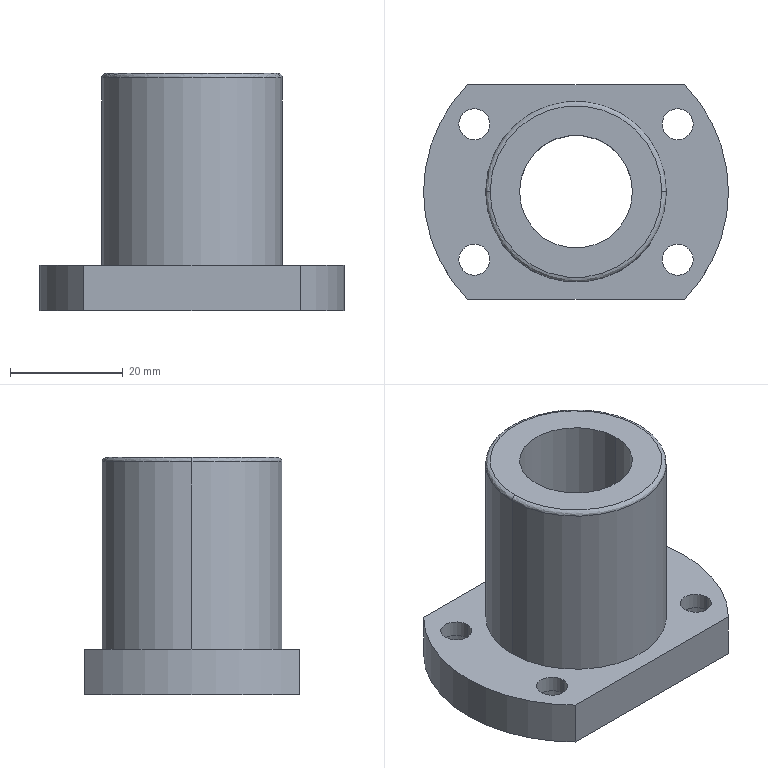Part | SolidWorks | features BaseBody 1 | 1 solid | 34 faces | box 54 x 38 x 42 mm | volume 27501 mm3 | cylinder 23 | plane 9 | spline 2 | commonest cylinder face diameters 5.5 x8 9 x8 54 x3 20 x2 32 x2
STEP:
#1=CARTESIAN_POINT('',(16.,0.,41.2));
#2=VERTEX_POINT('',#1);
#3=CARTESIAN_POINT('',(-16.,0.,41.2));
#4=VERTEX_POINT('',#3);
#5=CARTESIAN_POINT('',(0.,0.,41.2));
#6=DIRECTION('',(0.,0.,-1.));
#7=DIRECTION('',(1.,0.,0.));
#8=AXIS2_PLACEMENT_3D('',#5,#6,#7);
#9=CIRCLE('',#8,16.);
#10=EDGE_CURVE('',#2,#4,#9,.T.);
#11=ORIENTED_EDGE('',*,*,#10,.F.);
#12=CARTESIAN_POINT('',(15.2,0.,42.));
#13=VERTEX_POINT('',#12);
#14=CARTESIAN_POINT('',(15.2,0.,41.2));
#15=DIRECTION('',(0.,-1.,0.));
#16=DIRECTION('',(1.,0.,0.));
#17=AXIS2_PLACEMENT_3D('',#14,#15,#16);
#18=CIRCLE('',#17,0.8);
#19=EDGE_CURVE('',#2,#13,#18,.T.);
#20=ORIENTED_EDGE('',*,*,#19,.T.);
#21=CARTESIAN_POINT('',(-15.2,0.,42.));
#22=VERTEX_POINT('',#21);
#23=CARTESIAN_POINT('',(15.2,0.,42.));
#24=CARTESIAN_POINT('',(15.2,-30.4,42.));
#25=CARTESIAN_POINT('',(-15.2,-30.4,42.));
#26=CARTESIAN_POINT('',(-15.2,0.,42.));
#27=(BOUNDED_CURVE()B_SPLINE_CURVE(3,(#23,#24,#25,#26),.UNSPECIFIED.,.F.,.F.)B_SPLINE_CURVE_WITH_KNOTS((4,4),(0.5,1.),.UNSPECIFIED.)CURVE()GEOMETRIC_REPRESENTATION_ITEM()RATIONAL_B_SPLINE_CURVE((1.,0.3333,0.3333,1.))REPRESENTATION_ITEM(''));
#28=EDGE_CURVE('',#13,#22,#27,.T.);
#29=ORIENTED_EDGE('',*,*,#28,.T.);
#30=CARTESIAN_POINT('',(-15.2,0.,41.2));
#31=DIRECTION('',(0.,1.,0.));
#32=DIRECTION('',(-1.,0.,0.));
#33=AXIS2_PLACEMENT_3D('',#30,#31,#32);
#34=CIRCLE('',#33,0.8);
#35=EDGE_CURVE('',#4,#22,#34,.T.);
#36=ORIENTED_EDGE('',*,*,#35,.F.);
#37=EDGE_LOOP('',(#11,#20,#29,#36));
#38=FACE_OUTER_BOUND('',#37,.T.);
#39=CARTESIAN_POINT('',(16.,0.,41.2));
#40=CARTESIAN_POINT('',(16.,-32.,41.2));
#41=CARTESIAN_POINT('',(-16.,-32.,41.2));
#42=CARTESIAN_POINT('',(-16.,0.,41.2));
#43=CARTESIAN_POINT('',(16.,0.,41.669));
#44=CARTESIAN_POINT('',(16.,-32.,41.669));
#45=CARTESIAN_POINT('',(-16.,-32.,41.669));
#46=CARTESIAN_POINT('',(-16.,0.,41.669));
#47=CARTESIAN_POINT('',(15.669,0.,42.));
#48=CARTESIAN_POINT('',(15.669,-31.337,42.));
#49=CARTESIAN_POINT('',(-15.669,-31.337,42.));
#50=CARTESIAN_POINT('',(-15.669,0.,42.));
#51=CARTESIAN_POINT('',(15.2,0.,42.));
#52=CARTESIAN_POINT('',(15.2,-30.4,42.));
#53=CARTESIAN_POINT('',(-15.2,-30.4,42.));
#54=CARTESIAN_POINT('',(-15.2,0.,42.));
#55=(BOUNDED_SURFACE()B_SPLINE_SURFACE(3,3,((#39,#40,#41,#42),(#43,#44,#45,#46),(#47,#48,#49,#50),(#51,#52,#53,#54)),.UNSPECIFIED.,.F.,.F.,.F.)B_SPLINE_SURFACE_WITH_KNOTS((4,4),(4,4),(0.,1.),(0.,1.),.UNSPECIFIED.)GEOMETRIC_REPRESENTATION_ITEM()RATIONAL_B_SPLINE_SURFACE(((1.,0.3333,0.3333,1.),(0.8047,0.2682,0.2682,0.8047),(0.8047,0.2682,0.2682,0.8047),(1.,0.3333,0.3333,1.)))REPRESENTATION_ITEM('')SURFACE());
#56=ADVANCED_FACE('',(#38),#55,.T.);
#57=CARTESIAN_POINT('',(16.,0.,8.));
#58=VERTEX_POINT('',#57);
#59=CARTESIAN_POINT('',(-16.,0.,8.));
#60=VERTEX_POINT('',#59);
#61=CARTESIAN_POINT('',(0.,0.,8.));
#62=DIRECTION('',(0.,0.,1.));
#63=DIRECTION('',(1.,0.,0.));
#64=AXIS2_PLACEMENT_3D('',#61,#62,#63);
#65=CIRCLE('',#64,16.);
#66=EDGE_CURVE('',#58,#60,#65,.T.);
#67=ORIENTED_EDGE('',*,*,#66,.T.);
#68=CARTESIAN_POINT('',(-16.,0.,0.));
#69=DIRECTION('',(0.,0.,1.));
#70=VECTOR('',#69,1000.);
#71=LINE('',#68,#70);
#72=EDGE_CURVE('',#60,#4,#71,.T.);
#73=ORIENTED_EDGE('',*,*,#72,.T.);
#74=CARTESIAN_POINT('',(0.,0.,41.2));
#75=DIRECTION('',(0.,0.,-1.));
#76=DIRECTION('',(1.,0.,0.));
#77=AXIS2_PLACEMENT_3D('',#74,#75,#76);
#78=CIRCLE('',#77,16.);
#79=EDGE_CURVE('',#4,#2,#78,.T.);
#80=ORIENTED_EDGE('',*,*,#79,.T.);
#81=CARTESIAN_POINT('',(16.,0.,0.));
#82=DIRECTION('',(0.,0.,1.));
#83=VECTOR('',#82,1000.);
#84=LINE('',#81,#83);
#85=EDGE_CURVE('',#58,#2,#84,.T.);
#86=ORIENTED_EDGE('',*,*,#85,.F.);
#87=EDGE_LOOP('',(#67,#73,#80,#86));
#88=FACE_OUTER_BOUND('',#87,.T.);
#89=CARTESIAN_POINT('',(0.,0.,0.));
#90=DIRECTION('',(0.,0.,1.));
#91=DIRECTION('',(1.,0.,0.));
#92=AXIS2_PLACEMENT_3D('',#89,#90,#91);
#93=CYLINDRICAL_SURFACE('',#92,16.);
#94=ADVANCED_FACE('',(#88),#93,.T.);
#95=CARTESIAN_POINT('',(19.183,-19.,0.));
#96=VERTEX_POINT('',#95);
#97=CARTESIAN_POINT('',(27.,0.,0.));
#98=VERTEX_POINT('',#97);
#99=CARTESIAN_POINT('',(0.,0.,0.));
#100=DIRECTION('',(0.,0.,1.));
#101=DIRECTION('',(1.,0.,0.));
#102=AXIS2_PLACEMENT_3D('',#99,#100,#101);
#103=CIRCLE('',#102,27.);
#104=EDGE_CURVE('',#96,#98,#103,.T.);
#105=ORIENTED_EDGE('',*,*,#104,.T.);
#106=CARTESIAN_POINT('',(27.,0.,8.));
#107=VERTEX_POINT('',#106);
#108=CARTESIAN_POINT('',(27.,0.,8.));
#109=DIRECTION('',(0.,0.,1.));
#110=VECTOR('',#109,1000.);
#111=LINE('',#108,#110);
#112=EDGE_CURVE('',#98,#107,#111,.T.);
#113=ORIENTED_EDGE('',*,*,#112,.T.);
#114=CARTESIAN_POINT('',(19.183,-19.,8.));
#115=VERTEX_POINT('',#114);
#116=CARTESIAN_POINT('',(0.,0.,8.));
#117=DIRECTION('',(0.,0.,1.));
#118=DIRECTION('',(1.,0.,0.));
#119=AXIS2_PLACEMENT_3D('',#116,#117,#118);
#120=CIRCLE('',#119,27.);
#121=EDGE_CURVE('',#115,#107,#120,.T.);
#122=ORIENTED_EDGE('',*,*,#121,.F.);
#123=CARTESIAN_POINT('',(19.183,-19.,8.));
#124=DIRECTION('',(0.,0.,-1.));
#125=VECTOR('',#124,1000.);
#126=LINE('',#123,#125);
#127=EDGE_CURVE('',#115,#96,#126,.T.);
#128=ORIENTED_EDGE('',*,*,#127,.T.);
#129=EDGE_LOOP('',(#105,#113,#122,#128));
#130=FACE_OUTER_BOUND('',#129,.T.);
#131=CARTESIAN_POINT('',(0.,0.,8.));
#132=DIRECTION('',(0.,0.,1.));
#133=DIRECTION('',(1.,0.,0.));
#134=AXIS2_PLACEMENT_3D('',#131,#132,#133);
#135=CYLINDRICAL_SURFACE('',#134,27.);
#136=ADVANCED_FACE('',(#130),#135,.T.);
#137=CARTESIAN_POINT('',(-20.75,-12.,5.1));
#138=VERTEX_POINT('',#137);
#139=CARTESIAN_POINT('',(-15.25,-12.,5.1));
#140=VERTEX_POINT('',#139);
#141=CARTESIAN_POINT('',(-18.,-12.,5.1));
#142=DIRECTION('',(0.,0.,1.));
#143=DIRECTION('',(1.,0.,0.));
#144=AXIS2_PLACEMENT_3D('',#141,#142,#143);
#145=CIRCLE('',#144,2.75);
#146=EDGE_CURVE('',#138,#140,#145,.T.);
#147=ORIENTED_EDGE('',*,*,#146,.F.);
#148=CARTESIAN_POINT('',(-20.75,-12.,8.));
#149=VERTEX_POINT('',#148);
#150=CARTESIAN_POINT('',(-20.75,-12.,0.));
#151=DIRECTION('',(0.,0.,1.));
#152=VECTOR('',#151,1000.);
#153=LINE('',#150,#152);
#154=EDGE_CURVE('',#138,#149,#153,.T.);
#155=ORIENTED_EDGE('',*,*,#154,.T.);
#156=CARTESIAN_POINT('',(-15.25,-12.,8.));
#157=VERTEX_POINT('',#156);
#158=CARTESIAN_POINT('',(-18.,-12.,8.));
#159=DIRECTION('',(0.,0.,-1.));
#160=DIRECTION('',(1.,0.,0.));
#161=AXIS2_PLACEMENT_3D('',#158,#159,#160);
#162=CIRCLE('',#161,2.75);
#163=EDGE_CURVE('',#157,#149,#162,.T.);
#164=ORIENTED_EDGE('',*,*,#163,.F.);
#165=CARTESIAN_POINT('',(-15.25,-12.,0.));
#166=DIRECTION('',(0.,0.,1.));
#167=VECTOR('',#166,1000.);
#168=LINE('',#165,#167);
#169=EDGE_CURVE('',#140,#157,#168,.T.);
#170=ORIENTED_EDGE('',*,*,#169,.F.);
#171=EDGE_LOOP('',(#147,#155,#164,#170));
#172=FACE_OUTER_BOUND('',#171,.T.);
#173=CARTESIAN_POINT('',(-18.,-12.,0.));
#174=DIRECTION('',(0.,0.,1.));
#175=DIRECTION('',(1.,0.,0.));
#176=AXIS2_PLACEMENT_3D('',#173,#174,#175);
#177=CYLINDRICAL_SURFACE('',#176,2.75);
#178=ADVANCED_FACE('',(#172),#177,.F.);
#179=CARTESIAN_POINT('',(20.75,-12.,8.));
#180=VERTEX_POINT('',#179);
#181=CARTESIAN_POINT('',(15.25,-12.,8.));
#182=VERTEX_POINT('',#181);
#183=CARTESIAN_POINT('',(18.,-12.,8.));
#184=DIRECTION('',(0.,0.,-1.));
#185=DIRECTION('',(-1.,0.,0.));
#186=AXIS2_PLACEMENT_3D('',#183,#184,#185);
#187=CIRCLE('',#186,2.75);
#188=EDGE_CURVE('',#180,#182,#187,.T.);
#189=ORIENTED_EDGE('',*,*,#188,.F.);
#190=CARTESIAN_POINT('',(20.75,-12.,5.1));
#191=VERTEX_POINT('',#190);
#192=CARTESIAN_POINT('',(20.75,-12.,8.));
#193=DIRECTION('',(0.,0.,-1.));
#194=VECTOR('',#193,1000.);
#195=LINE('',#192,#194);
#196=EDGE_CURVE('',#180,#191,#195,.T.);
#197=ORIENTED_EDGE('',*,*,#196,.T.);
#198=CARTESIAN_POINT('',(15.25,-12.,5.1));
#199=VERTEX_POINT('',#198);
#200=CARTESIAN_POINT('',(18.,-12.,5.1));
#201=DIRECTION('',(0.,0.,1.));
#202=DIRECTION('',(-1.,0.,0.));
#203=AXIS2_PLACEMENT_3D('',#200,#201,#202);
#204=CIRCLE('',#203,2.75);
#205=EDGE_CURVE('',#199,#191,#204,.T.);
#206=ORIENTED_EDGE('',*,*,#205,.F.);
#207=CARTESIAN_POINT('',(15.25,-12.,8.));
#208=DIRECTION('',(0.,0.,-1.));
#209=VECTOR('',#208,1000.);
#210=LINE('',#207,#209);
#211=EDGE_CURVE('',#182,#199,#210,.T.);
#212=ORIENTED_EDGE('',*,*,#211,.F.);
#213=EDGE_LOOP('',(#189,#197,#206,#212));
#214=FACE_OUTER_BOUND('',#213,.T.);
#215=CARTESIAN_POINT('',(18.,-12.,8.));
#216=DIRECTION('',(0.,0.,-1.));
#217=DIRECTION('',(-1.,0.,0.));
#218=AXIS2_PLACEMENT_3D('',#215,#216,#217);
#219=CYLINDRICAL_SURFACE('',#218,2.75);
#220=ADVANCED_FACE('',(#214),#219,.F.);
#221=CARTESIAN_POINT('',(-20.75,12.,5.1));
#222=VERTEX_POINT('',#221);
#223=CARTESIAN_POINT('',(-15.25,12.,5.1));
#224=VERTEX_POINT('',#223);
#225=CARTESIAN_POINT('',(-18.,12.,5.1));
#226=DIRECTION('',(0.,0.,1.));
#227=DIRECTION('',(1.,0.,0.));
#228=AXIS2_PLACEMENT_3D('',#225,#226,#227);
#229=CIRCLE('',#228,2.75);
#230=EDGE_CURVE('',#222,#224,#229,.T.);
#231=ORIENTED_EDGE('',*,*,#230,.F.);
#232=CARTESIAN_POINT('',(-20.75,12.,8.));
#233=VERTEX_POINT('',#232);
#234=CARTESIAN_POINT('',(-20.75,12.,0.));
#235=DIRECTION('',(0.,0.,1.));
#236=VECTOR('',#235,1000.);
#237=LINE('',#234,#236);
#238=EDGE_CURVE('',#222,#233,#237,.T.);
#239=ORIENTED_EDGE('',*,*,#238,.T.);
#240=CARTESIAN_POINT('',(-15.25,12.,8.));
#241=VERTEX_POINT('',#240);
#242=CARTESIAN_POINT('',(-18.,12.,8.));
#243=DIRECTION('',(0.,0.,-1.));
#244=DIRECTION('',(1.,0.,0.));
#245=AXIS2_PLACEMENT_3D('',#242,#243,#244);
#246=CIRCLE('',#245,2.75);
#247=EDGE_CURVE('',#241,#233,#246,.T.);
#248=ORIENTED_EDGE('',*,*,#247,.F.);
#249=CARTESIAN_POINT('',(-15.25,12.,0.));
#250=DIRECTION('',(0.,0.,1.));
#251=VECTOR('',#250,1000.);
#252=LINE('',#249,#251);
#253=EDGE_CURVE('',#224,#241,#252,.T.);
#254=ORIENTED_EDGE('',*,*,#253,.F.);
#255=EDGE_LOOP('',(#231,#239,#248,#254));
#256=FACE_OUTER_BOUND('',#255,.T.);
#257=CARTESIAN_POINT('',(-18.,12.,0.));
#258=DIRECTION('',(0.,0.,1.));
#259=DIRECTION('',(1.,0.,0.));
#260=AXIS2_PLACEMENT_3D('',#257,#258,#259);
#261=CYLINDRICAL_SURFACE('',#260,2.75);
#262=ADVANCED_FACE('',(#256),#261,.F.);
#263=CARTESIAN_POINT('',(20.75,12.,8.));
#264=VERTEX_POINT('',#263);
#265=CARTESIAN_POINT('',(15.25,12.,8.));
#266=VERTEX_POINT('',#265);
#267=CARTESIAN_POINT('',(18.,12.,8.));
#268=DIRECTION('',(0.,0.,-1.));
#269=DIRECTION('',(-1.,0.,0.));
#270=AXIS2_PLACEMENT_3D('',#267,#268,#269);
#271=CIRCLE('',#270,2.75);
#272=EDGE_CURVE('',#264,#266,#271,.T.);
#273=ORIENTED_EDGE('',*,*,#272,.F.);
#274=CARTESIAN_POINT('',(20.75,12.,5.1));
#275=VERTEX_POINT('',#274);
#276=CARTESIAN_POINT('',(20.75,12.,8.));
#277=DIRECTION('',(0.,0.,-1.));
#278=VECTOR('',#277,1000.);
#279=LINE('',#276,#278);
#280=EDGE_CURVE('',#264,#275,#279,.T.);
#281=ORIENTED_EDGE('',*,*,#280,.T.);
#282=CARTESIAN_POINT('',(15.25,12.,5.1));
#283=VERTEX_POINT('',#282);
#284=CARTESIAN_POINT('',(18.,12.,5.1));
#285=DIRECTION('',(0.,0.,1.));
#286=DIRECTION('',(-1.,0.,0.));
#287=AXIS2_PLACEMENT_3D('',#284,#285,#286);
#288=CIRCLE('',#287,2.75);
#289=EDGE_CURVE('',#283,#275,#288,.T.);
#290=ORIENTED_EDGE('',*,*,#289,.F.);
#291=CARTESIAN_POINT('',(15.25,12.,8.));
#292=DIRECTION('',(0.,0.,-1.));
#293=VECTOR('',#292,1000.);
#294=LINE('',#291,#293);
#295=EDGE_CURVE('',#266,#283,#294,.T.);
#296=ORIENTED_EDGE('',*,*,#295,.F.);
#297=EDGE_LOOP('',(#273,#281,#290,#296));
#298=FACE_OUTER_BOUND('',#297,.T.);
#299=CARTESIAN_POINT('',(18.,12.,8.));
#300=DIRECTION('',(0.,0.,-1.));
#301=DIRECTION('',(-1.,0.,0.));
#302=AXIS2_PLACEMENT_3D('',#299,#300,#301);
#303=CYLINDRICAL_SURFACE('',#302,2.75);
#304=ADVANCED_FACE('',(#298),#303,.F.);
#305=CARTESIAN_POINT('',(-10.,0.,0.));
#306=VERTEX_POINT('',#305);
#307=CARTESIAN_POINT('',(10.,0.,0.));
#308=VERTEX_POINT('',#307);
#309=CARTESIAN_POINT('',(0.,0.,0.));
#310=DIRECTION('',(0.,0.,1.));
#311=DIRECTION('',(1.,0.,0.));
#312=AXIS2_PLACEMENT_3D('',#309,#310,#311);
#313=CIRCLE('',#312,10.);
#314=EDGE_CURVE('',#306,#308,#313,.T.);
#315=ORIENTED_EDGE('',*,*,#314,.F.);
#316=CARTESIAN_POINT('',(-10.,0.,42.));
#317=VERTEX_POINT('',#316);
#318=CARTESIAN_POINT('',(-10.,0.,0.));
#319=DIRECTION('',(0.,0.,1.));
#320=VECTOR('',#319,1000.);
#321=LINE('',#318,#320);
#322=EDGE_CURVE('',#306,#317,#321,.T.);
#323=ORIENTED_EDGE('',*,*,#322,.T.);
#324=CARTESIAN_POINT('',(10.,0.,42.));
#325=VERTEX_POINT('',#324);
#326=CARTESIAN_POINT('',(0.,0.,42.));
#327=DIRECTION('',(0.,0.,-1.));
#328=DIRECTION('',(1.,0.,0.));
#329=AXIS2_PLACEMENT_3D('',#326,#327,#328);
#330=CIRCLE('',#329,10.);
#331=EDGE_CURVE('',#325,#317,#330,.T.);
#332=ORIENTED_EDGE('',*,*,#331,.F.);
#333=CARTESIAN_POINT('',(10.,0.,0.));
#334=DIRECTION('',(0.,0.,1.));
#335=VECTOR('',#334,1000.);
#336=LINE('',#333,#335);
#337=EDGE_CURVE('',#308,#325,#336,.T.);
#338=ORIENTED_EDGE('',*,*,#337,.F.);
#339=EDGE_LOOP('',(#315,#323,#332,#338));
#340=FACE_OUTER_BOUND('',#339,.T.);
#341=CARTESIAN_POINT('',(0.,0.,0.));
#342=DIRECTION('',(0.,0.,1.));
#343=DIRECTION('',(1.,0.,0.));
#344=AXIS2_PLACEMENT_3D('',#341,#342,#343);
#345=CYLINDRICAL_SURFACE('',#344,10.);
#346=ADVANCED_FACE('',(#340),#345,.F.);
#347=CARTESIAN_POINT('',(-22.5,-12.,0.));
#348=VERTEX_POINT('',#347);
#349=CARTESIAN_POINT('',(-13.5,-12.,0.));
#350=VERTEX_POINT('',#349);
#351=CARTESIAN_POINT('',(-18.,-12.,0.));
#352=DIRECTION('',(0.,0.,1.));
#353=DIRECTION('',(1.,0.,0.));
#354=AXIS2_PLACEMENT_3D('',#351,#352,#353);
#355=CIRCLE('',#354,4.5);
#356=EDGE_CURVE('',#348,#350,#355,.T.);
#357=ORIENTED_EDGE('',*,*,#356,.F.);
#358=CARTESIAN_POINT('',(-22.5,-12.,5.1));
#359=VERTEX_POINT('',#358);
#360=CARTESIAN_POINT('',(-22.5,-12.,0.));
#361=DIRECTION('',(0.,0.,1.));
#362=VECTOR('',#361,1000.);
#363=LINE('',#360,#362);
#364=EDGE_CURVE('',#348,#359,#363,.T.);
#365=ORIENTED_EDGE('',*,*,#364,.T.);
#366=CARTESIAN_POINT('',(-13.5,-12.,5.1));
#367=VERTEX_POINT('',#366);
#368=CARTESIAN_POINT('',(-18.,-12.,5.1));
#369=DIRECTION('',(0.,0.,-1.));
#370=DIRECTION('',(1.,0.,0.));
#371=AXIS2_PLACEMENT_3D('',#368,#369,#370);
#372=CIRCLE('',#371,4.5);
#373=EDGE_CURVE('',#367,#359,#372,.T.);
#374=ORIENTED_EDGE('',*,*,#373,.F.);
#375=CARTESIAN_POINT('',(-13.5,-12.,0.));
#376=DIRECTION('',(0.,0.,1.));
#377=VECTOR('',#376,1000.);
#378=LINE('',#375,#377);
#379=EDGE_CURVE('',#350,#367,#378,.T.);
#380=ORIENTED_EDGE('',*,*,#379,.F.);
#381=EDGE_LOOP('',(#357,#365,#374,#380));
#382=FACE_OUTER_BOUND('',#381,.T.);
#383=CARTESIAN_POINT('',(-18.,-12.,0.));
#384=DIRECTION('',(0.,0.,1.));
#385=DIRECTION('',(1.,0.,0.));
#386=AXIS2_PLACEMENT_3D('',#383,#384,#385);
#387=CYLINDRICAL_SURFACE('',#386,4.5);
#388=ADVANCED_FACE('',(#382),#387,.F.);
#389=CARTESIAN_POINT('',(22.5,-12.,5.1));
#390=VERTEX_POINT('',#389);
#391=CARTESIAN_POINT('',(13.5,-12.,5.1));
#392=VERTEX_POINT('',#391);
#393=CARTESIAN_POINT('',(18.,-12.,5.1));
#394=DIRECTION('',(0.,0.,-1.));
#395=DIRECTION('',(-1.,0.,0.));
#396=AXIS2_PLACEMENT_3D('',#393,#394,#395);
#397=CIRCLE('',#396,4.5);
#398=EDGE_CURVE('',#390,#392,#397,.T.);
#399=ORIENTED_EDGE('',*,*,#398,.F.);
#400=CARTESIAN_POINT('',(22.5,-12.,0.));
#401=VERTEX_POINT('',#400);
#402=CARTESIAN_POINT('',(22.5,-12.,8.));
#403=DIRECTION('',(0.,0.,-1.));
#404=VECTOR('',#403,1000.);
#405=LINE('',#402,#404);
#406=EDGE_CURVE('',#390,#401,#405,.T.);
#407=ORIENTED_EDGE('',*,*,#406,.T.);
#408=CARTESIAN_POINT('',(13.5,-12.,0.));
#409=VERTEX_POINT('',#408);
#410=CARTESIAN_POINT('',(18.,-12.,0.));
#411=DIRECTION('',(0.,0.,1.));
#412=DIRECTION('',(-1.,0.,0.));
#413=AXIS2_PLACEMENT_3D('',#410,#411,#412);
#414=CIRCLE('',#413,4.5);
#415=EDGE_CURVE('',#409,#401,#414,.T.);
#416=ORIENTED_EDGE('',*,*,#415,.F.);
#417=CARTESIAN_POINT('',(13.5,-12.,8.));
#418=DIRECTION('',(0.,0.,-1.));
#419=VECTOR('',#418,1000.);
#420=LINE('',#417,#419);
#421=EDGE_CURVE('',#392,#409,#420,.T.);
#422=ORIENTED_EDGE('',*,*,#421,.F.);
#423=EDGE_LOOP('',(#399,#407,#416,#422));
#424=FACE_OUTER_BOUND('',#423,.T.);
#425=CARTESIAN_POINT('',(18.,-12.,8.));
#426=DIRECTION('',(0.,0.,-1.));
#427=DIRECTION('',(-1.,0.,0.));
#428=AXIS2_PLACEMENT_3D('',#425,#426,#427);
#429=CYLINDRICAL_SURFACE('',#428,4.5);
#430=ADVANCED_FACE('',(#424),#429,.F.);
#431=CARTESIAN_POINT('',(-22.5,12.,0.));
#432=VERTEX_POINT('',#431);
#433=CARTESIAN_POINT('',(-13.5,12.,0.));
#434=VERTEX_POINT('',#433);
#435=CARTESIAN_POINT('',(-18.,12.,0.));
#436=DIRECTION('',(0.,0.,1.));
#437=DIRECTION('',(1.,0.,0.));
#438=AXIS2_PLACEMENT_3D('',#435,#436,#437);
#439=CIRCLE('',#438,4.5);
#440=EDGE_CURVE('',#432,#434,#439,.T.);
#441=ORIENTED_EDGE('',*,*,#440,.F.);
#442=CARTESIAN_POINT('',(-22.5,12.,5.1));
#443=VERTEX_POINT('',#442);
#444=CARTESIAN_POINT('',(-22.5,12.,0.));
#445=DIRECTION('',(0.,0.,1.));
#446=VECTOR('',#445,1000.);
#447=LINE('',#444,#446);
#448=EDGE_CURVE('',#432,#443,#447,.T.);
#449=ORIENTED_EDGE('',*,*,#448,.T.);
#450=CARTESIAN_POINT('',(-13.5,12.,5.1));
#451=VERTEX_POINT('',#450);
#452=CARTESIAN_POINT('',(-18.,12.,5.1));
#453=DIRECTION('',(0.,0.,-1.));
#454=DIRECTION('',(1.,0.,0.));
#455=AXIS2_PLACEMENT_3D('',#452,#453,#454);
#456=CIRCLE('',#455,4.5);
#457=EDGE_CURVE('',#451,#443,#456,.T.);
#458=ORIENTED_EDGE('',*,*,#457,.F.);
#459=CARTESIAN_POINT('',(-13.5,12.,0.));
#460=DIRECTION('',(0.,0.,1.));
#461=VECTOR('',#460,1000.);
#462=LINE('',#459,#461);
#463=EDGE_CURVE('',#434,#451,#462,.T.);
#464=ORIENTED_EDGE('',*,*,#463,.F.);
#465=EDGE_LOOP('',(#441,#449,#458,#464));
#466=FACE_OUTER_BOUND('',#465,.T.);
#467=CARTESIAN_POINT('',(-18.,12.,0.));
#468=DIRECTION('',(0.,0.,1.));
#469=DIRECTION('',(1.,0.,0.));
#470=AXIS2_PLACEMENT_3D('',#467,#468,#469);
#471=CYLINDRICAL_SURFACE('',#470,4.5);
#472=ADVANCED_FACE('',(#466),#471,.F.);
#473=CARTESIAN_POINT('',(22.5,12.,5.1));
#474=VERTEX_POINT('',#473);
#475=CARTESIAN_POINT('',(13.5,12.,5.1));
#476=VERTEX_POINT('',#475);
#477=CARTESIAN_POINT('',(18.,12.,5.1));
#478=DIRECTION('',(0.,0.,-1.));
#479=DIRECTION('',(-1.,0.,0.));
#480=AXIS2_PLACEMENT_3D('',#477,#478,#479);
#481=CIRCLE('',#480,4.5);
#482=EDGE_CURVE('',#474,#476,#481,.T.);
#483=ORIENTED_EDGE('',*,*,#482,.F.);
#484=CARTESIAN_POINT('',(22.5,12.,0.));
#485=VERTEX_POINT('',#484);
#486=CARTESIAN_POINT('',(22.5,12.,8.));
#487=DIRECTION('',(0.,0.,-1.));
#488=VECTOR('',#487,1000.);
#489=LINE('',#486,#488);
#490=EDGE_CURVE('',#474,#485,#489,.T.);
#491=ORIENTED_EDGE('',*,*,#490,.T.);
#492=CARTESIAN_POINT('',(13.5,12.,0.));
#493=VERTEX_POINT('',#492);
#494=CARTESIAN_POINT('',(18.,12.,0.));
#495=DIRECTION('',(0.,0.,1.));
#496=DIRECTION('',(-1.,0.,0.));
#497=AXIS2_PLACEMENT_3D('',#494,#495,#496);
#498=CIRCLE('',#497,4.5);
#499=EDGE_CURVE('',#493,#485,#498,.T.);
#500=ORIENTED_EDGE('',*,*,#499,.F.);
#501=CARTESIAN_POINT('',(13.5,12.,8.));
#502=DIRECTION('',(0.,0.,-1.));
#503=VECTOR('',#502,1000.);
#504=LINE('',#501,#503);
#505=EDGE_CURVE('',#476,#493,#504,.T.);
#506=ORIENTED_EDGE('',*,*,#505,.F.);
#507=EDGE_LOOP('',(#483,#491,#500,#506));
#508=FACE_OUTER_BOUND('',#507,.T.);
#509=CARTESIAN_POINT('',(18.,12.,8.));
#510=DIRECTION('',(0.,0.,-1.));
#511=DIRECTION('',(-1.,0.,0.));
#512=AXIS2_PLACEMENT_3D('',#509,#510,#511);
#513=CYLINDRICAL_SURFACE('',#512,4.5);
#514=ADVANCED_FACE('',(#508),#513,.F.);
#515=ORIENTED_EDGE('',*,*,#72,.F.);
#516=CARTESIAN_POINT('',(0.,0.,8.));
#517=DIRECTION('',(0.,0.,1.));
#518=DIRECTION('',(1.,0.,0.));
#519=AXIS2_PLACEMENT_3D('',#516,#517,#518);
#520=CIRCLE('',#519,16.);
#521=EDGE_CURVE('',#60,#58,#520,.T.);
#522=ORIENTED_EDGE('',*,*,#521,.T.);
#523=ORIENTED_EDGE('',*,*,#85,.T.);
#524=ORIENTED_EDGE('',*,*,#10,.T.);
#525=EDGE_LOOP('',(#515,#522,#523,#524));
#526=FACE_OUTER_BOUND('',#525,.T.);
#527=CARTESIAN_POINT('',(0.,0.,0.));
#528=DIRECTION('',(0.,0.,1.));
#529=DIRECTION('',(1.,0.,0.));
#530=AXIS2_PLACEMENT_3D('',#527,#528,#529);
#531=CYLINDRICAL_SURFACE('',#530,16.);
#532=ADVANCED_FACE('',(#526),#531,.T.);
#533=CARTESIAN_POINT('',(-19.183,-19.,8.));
#534=VERTEX_POINT('',#533);
#535=CARTESIAN_POINT('',(0.,-19.,8.));
#536=DIRECTION('',(1.,0.,0.));
#537=VECTOR('',#536,1000.);
#538=LINE('',#535,#537);
#539=EDGE_CURVE('',#534,#115,#538,.T.);
#540=ORIENTED_EDGE('',*,*,#539,.T.);
#541=ORIENTED_EDGE('',*,*,#121,.T.);
#542=CARTESIAN_POINT('',(19.183,19.,8.));
#543=VERTEX_POINT('',#542);
#544=CARTESIAN_POINT('',(0.,0.,8.));
#545=DIRECTION('',(0.,0.,1.));
#546=DIRECTION('',(1.,0.,0.));
#547=AXIS2_PLACEMENT_3D('',#544,#545,#546);
#548=CIRCLE('',#547,27.);
#549=EDGE_CURVE('',#107,#543,#548,.T.);
#550=ORIENTED_EDGE('',*,*,#549,.T.);
#551=CARTESIAN_POINT('',(-19.183,19.,8.));
#552=VERTEX_POINT('',#551);
#553=CARTESIAN_POINT('',(0.,19.,8.));
#554=DIRECTION('',(-1.,0.,0.));
#555=VECTOR('',#554,1000.);
#556=LINE('',#553,#555);
#557=EDGE_CURVE('',#543,#552,#556,.T.);
#558=ORIENTED_EDGE('',*,*,#557,.T.);
#559=CARTESIAN_POINT('',(0.,0.,8.));
#560=DIRECTION('',(0.,0.,1.));
#561=DIRECTION('',(1.,0.,0.));
#562=AXIS2_PLACEMENT_3D('',#559,#560,#561);
#563=CIRCLE('',#562,27.);
#564=EDGE_CURVE('',#552,#534,#563,.T.);
#565=ORIENTED_EDGE('',*,*,#564,.T.);
#566=EDGE_LOOP('',(#540,#541,#550,#558,#565));
#567=FACE_OUTER_BOUND('',#566,.T.);
#568=ORIENTED_EDGE('',*,*,#66,.F.);
#569=ORIENTED_EDGE('',*,*,#521,.F.);
#570=EDGE_LOOP('',(#568,#569));
#571=FACE_BOUND('',#570,.T.);
#572=ORIENTED_EDGE('',*,*,#163,.T.);
#573=CARTESIAN_POINT('',(-18.,-12.,8.));
#574=DIRECTION('',(0.,0.,-1.));
#575=DIRECTION('',(1.,0.,0.));
#576=AXIS2_PLACEMENT_3D('',#573,#574,#575);
#577=CIRCLE('',#576,2.75);
#578=EDGE_CURVE('',#149,#157,#577,.T.);
#579=ORIENTED_EDGE('',*,*,#578,.T.);
#580=EDGE_LOOP('',(#572,#579));
#581=FACE_BOUND('',#580,.T.);
#582=CARTESIAN_POINT('',(18.,-12.,8.));
#583=DIRECTION('',(0.,0.,-1.));
#584=DIRECTION('',(-1.,0.,0.));
#585=AXIS2_PLACEMENT_3D('',#582,#583,#584);
#586=CIRCLE('',#585,2.75);
#587=EDGE_CURVE('',#182,#180,#586,.T.);
#588=ORIENTED_EDGE('',*,*,#587,.T.);
#589=ORIENTED_EDGE('',*,*,#188,.T.);
#590=EDGE_LOOP('',(#588,#589));
#591=FACE_BOUND('',#590,.T.);
#592=ORIENTED_EDGE('',*,*,#247,.T.);
#593=CARTESIAN_POINT('',(-18.,12.,8.));
#594=DIRECTION('',(0.,0.,-1.));
#595=DIRECTION('',(1.,0.,0.));
#596=AXIS2_PLACEMENT_3D('',#593,#594,#595);
#597=CIRCLE('',#596,2.75);
#598=EDGE_CURVE('',#233,#241,#597,.T.);
#599=ORIENTED_EDGE('',*,*,#598,.T.);
#600=EDGE_LOOP('',(#592,#599));
#601=FACE_BOUND('',#600,.T.);
#602=CARTESIAN_POINT('',(18.,12.,8.));
#603=DIRECTION('',(0.,0.,-1.));
#604=DIRECTION('',(-1.,0.,0.));
#605=AXIS2_PLACEMENT_3D('',#602,#603,#604);
#606=CIRCLE('',#605,2.75);
#607=EDGE_CURVE('',#266,#264,#606,.T.);
#608=ORIENTED_EDGE('',*,*,#607,.T.);
#609=ORIENTED_EDGE('',*,*,#272,.T.);
#610=EDGE_LOOP('',(#608,#609));
#611=FACE_BOUND('',#610,.T.);
#612=CARTESIAN_POINT('',(0.,0.,8.));
#613=DIRECTION('',(0.,0.,1.));
#614=DIRECTION('',(1.,0.,0.));
#615=AXIS2_PLACEMENT_3D('',#612,#613,#614);
#616=PLANE('',#615);
#617=ADVANCED_FACE('',(#567,#571,#581,#591,#601,#611),#616,.T.);
#618=ORIENTED_EDGE('',*,*,#19,.F.);
#619=ORIENTED_EDGE('',*,*,#79,.F.);
#620=ORIENTED_EDGE('',*,*,#35,.T.);
#621=CARTESIAN_POINT('',(-15.2,0.,42.));
#622=CARTESIAN_POINT('',(-15.2,30.4,42.));
#623=CARTESIAN_POINT('',(15.2,30.4,42.));
#624=CARTESIAN_POINT('',(15.2,0.,42.));
#625=(BOUNDED_CURVE()B_SPLINE_CURVE(3,(#621,#622,#623,#624),.UNSPECIFIED.,.F.,.T.)B_SPLINE_CURVE_WITH_KNOTS((4,4),(0.,0.5),.UNSPECIFIED.)CURVE()GEOMETRIC_REPRESENTATION_ITEM()RATIONAL_B_SPLINE_CURVE((1.,0.3333,0.3333,1.))REPRESENTATION_ITEM(''));
#626=EDGE_CURVE('',#22,#13,#625,.T.);
#627=ORIENTED_EDGE('',*,*,#626,.T.);
#628=EDGE_LOOP('',(#618,#619,#620,#627));
#629=FACE_OUTER_BOUND('',#628,.T.);
#630=CARTESIAN_POINT('',(-16.,0.,41.2));
#631=CARTESIAN_POINT('',(-16.,32.,41.2));
#632=CARTESIAN_POINT('',(16.,32.,41.2));
#633=CARTESIAN_POINT('',(16.,0.,41.2));
#634=CARTESIAN_POINT('',(-16.,0.,41.669));
#635=CARTESIAN_POINT('',(-16.,32.,41.669));
#636=CARTESIAN_POINT('',(16.,32.,41.669));
#637=CARTESIAN_POINT('',(16.,0.,41.669));
#638=CARTESIAN_POINT('',(-15.669,0.,42.));
#639=CARTESIAN_POINT('',(-15.669,31.337,42.));
#640=CARTESIAN_POINT('',(15.669,31.337,42.));
#641=CARTESIAN_POINT('',(15.669,0.,42.));
#642=CARTESIAN_POINT('',(-15.2,0.,42.));
#643=CARTESIAN_POINT('',(-15.2,30.4,42.));
#644=CARTESIAN_POINT('',(15.2,30.4,42.));
#645=CARTESIAN_POINT('',(15.2,0.,42.));
#646=(BOUNDED_SURFACE()B_SPLINE_SURFACE(3,3,((#630,#631,#632,#633),(#634,#635,#636,#637),(#638,#639,#640,#641),(#642,#643,#644,#645)),.UNSPECIFIED.,.F.,.F.,.F.)B_SPLINE_SURFACE_WITH_KNOTS((4,4),(4,4),(0.,1.),(0.,1.),.UNSPECIFIED.)GEOMETRIC_REPRESENTATION_ITEM()RATIONAL_B_SPLINE_SURFACE(((1.,0.3333,0.3333,1.),(0.8047,0.2682,0.2682,0.8047),(0.8047,0.2682,0.2682,0.8047),(1.,0.3333,0.3333,1.)))REPRESENTATION_ITEM('')SURFACE());
#647=ADVANCED_FACE('',(#629),#646,.T.);
#648=ORIENTED_EDGE('',*,*,#112,.F.);
#649=CARTESIAN_POINT('',(19.183,19.,0.));
#650=VERTEX_POINT('',#649);
#651=CARTESIAN_POINT('',(0.,0.,0.));
#652=DIRECTION('',(0.,0.,1.));
#653=DIRECTION('',(1.,0.,0.));
#654=AXIS2_PLACEMENT_3D('',#651,#652,#653);
#655=CIRCLE('',#654,27.);
#656=EDGE_CURVE('',#98,#650,#655,.T.);
#657=ORIENTED_EDGE('',*,*,#656,.T.);
#658=CARTESIAN_POINT('',(19.183,19.,8.));
#659=DIRECTION('',(0.,0.,1.));
#660=VECTOR('',#659,1000.);
#661=LINE('',#658,#660);
#662=EDGE_CURVE('',#650,#543,#661,.T.);
#663=ORIENTED_EDGE('',*,*,#662,.T.);
#664=ORIENTED_EDGE('',*,*,#549,.F.);
#665=EDGE_LOOP('',(#648,#657,#663,#664));
#666=FACE_OUTER_BOUND('',#665,.T.);
#667=CARTESIAN_POINT('',(0.,0.,8.));
#668=DIRECTION('',(0.,0.,1.));
#669=DIRECTION('',(1.,0.,0.));
#670=AXIS2_PLACEMENT_3D('',#667,#668,#669);
#671=CYLINDRICAL_SURFACE('',#670,27.);
#672=ADVANCED_FACE('',(#666),#671,.T.);
#673=ORIENTED_EDGE('',*,*,#127,.F.);
#674=ORIENTED_EDGE('',*,*,#539,.F.);
#675=CARTESIAN_POINT('',(-19.183,-19.,0.));
#676=VERTEX_POINT('',#675);
#677=CARTESIAN_POINT('',(-19.183,-19.,8.));
#678=DIRECTION('',(0.,0.,1.));
#679=VECTOR('',#678,1000.);
#680=LINE('',#677,#679);
#681=EDGE_CURVE('',#676,#534,#680,.T.);
#682=ORIENTED_EDGE('',*,*,#681,.F.);
#683=CARTESIAN_POINT('',(-19.183,-19.,0.));
#684=DIRECTION('',(-1.,0.,0.));
#685=VECTOR('',#684,1000.);
#686=LINE('',#683,#685);
#687=EDGE_CURVE('',#96,#676,#686,.T.);
#688=ORIENTED_EDGE('',*,*,#687,.F.);
#689=EDGE_LOOP('',(#673,#674,#682,#688));
#690=FACE_OUTER_BOUND('',#689,.T.);
#691=CARTESIAN_POINT('',(-19.183,-19.,8.));
#692=DIRECTION('',(0.,1.,0.));
#693=DIRECTION('',(0.,0.,1.));
#694=AXIS2_PLACEMENT_3D('',#691,#692,#693);
#695=PLANE('',#694);
#696=ADVANCED_FACE('',(#690),#695,.F.);
#697=ORIENTED_EDGE('',*,*,#564,.F.);
#698=CARTESIAN_POINT('',(-19.183,19.,0.));
#699=VERTEX_POINT('',#698);
#700=CARTESIAN_POINT('',(-19.183,19.,8.));
#701=DIRECTION('',(0.,0.,-1.));
#702=VECTOR('',#701,1000.);
#703=LINE('',#700,#702);
#704=EDGE_CURVE('',#552,#699,#703,.T.);
#705=ORIENTED_EDGE('',*,*,#704,.T.);
#706=CARTESIAN_POINT('',(0.,0.,0.));
#707=DIRECTION('',(0.,0.,1.));
#708=DIRECTION('',(1.,0.,0.));
#709=AXIS2_PLACEMENT_3D('',#706,#707,#708);
#710=CIRCLE('',#709,27.);
#711=EDGE_CURVE('',#699,#676,#710,.T.);
#712=ORIENTED_EDGE('',*,*,#711,.T.);
#713=ORIENTED_EDGE('',*,*,#681,.T.);
#714=EDGE_LOOP('',(#697,#705,#712,#713));
#715=FACE_OUTER_BOUND('',#714,.T.);
#716=CARTESIAN_POINT('',(0.,0.,8.));
#717=DIRECTION('',(0.,0.,1.));
#718=DIRECTION('',(1.,0.,0.));
#719=AXIS2_PLACEMENT_3D('',#716,#717,#718);
#720=CYLINDRICAL_SURFACE('',#719,27.);
#721=ADVANCED_FACE('',(#715),#720,.T.);
#722=ORIENTED_EDGE('',*,*,#704,.F.);
#723=ORIENTED_EDGE('',*,*,#557,.F.);
#724=ORIENTED_EDGE('',*,*,#662,.F.);
#725=CARTESIAN_POINT('',(19.183,19.,0.));
#726=DIRECTION('',(1.,0.,0.));
#727=VECTOR('',#726,1000.);
#728=LINE('',#725,#727);
#729=EDGE_CURVE('',#699,#650,#728,.T.);
#730=ORIENTED_EDGE('',*,*,#729,.F.);
#731=EDGE_LOOP('',(#722,#723,#724,#730));
#732=FACE_OUTER_BOUND('',#731,.T.);
#733=CARTESIAN_POINT('',(19.183,19.,8.));
#734=DIRECTION('',(0.,-1.,0.));
#735=DIRECTION('',(0.,0.,-1.));
#736=AXIS2_PLACEMENT_3D('',#733,#734,#735);
#737=PLANE('',#736);
#738=ADVANCED_FACE('',(#732),#737,.F.);
#739=ORIENTED_EDGE('',*,*,#154,.F.);
#740=CARTESIAN_POINT('',(-18.,-12.,5.1));
#741=DIRECTION('',(0.,0.,1.));
#742=DIRECTION('',(1.,0.,0.));
#743=AXIS2_PLACEMENT_3D('',#740,#741,#742);
#744=CIRCLE('',#743,2.75);
#745=EDGE_CURVE('',#140,#138,#744,.T.);
#746=ORIENTED_EDGE('',*,*,#745,.F.);
#747=ORIENTED_EDGE('',*,*,#169,.T.);
#748=ORIENTED_EDGE('',*,*,#578,.F.);
#749=EDGE_LOOP('',(#739,#746,#747,#748));
#750=FACE_OUTER_BOUND('',#749,.T.);
#751=CARTESIAN_POINT('',(-18.,-12.,0.));
#752=DIRECTION('',(0.,0.,1.));
#753=DIRECTION('',(1.,0.,0.));
#754=AXIS2_PLACEMENT_3D('',#751,#752,#753);
#755=CYLINDRICAL_SURFACE('',#754,2.75);
#756=ADVANCED_FACE('',(#750),#755,.F.);
#757=ORIENTED_EDGE('',*,*,#196,.F.);
#758=ORIENTED_EDGE('',*,*,#587,.F.);
#759=ORIENTED_EDGE('',*,*,#211,.T.);
#760=CARTESIAN_POINT('',(18.,-12.,5.1));
#761=DIRECTION('',(0.,0.,1.));
#762=DIRECTION('',(-1.,0.,0.));
#763=AXIS2_PLACEMENT_3D('',#760,#761,#762);
#764=CIRCLE('',#763,2.75);
#765=EDGE_CURVE('',#191,#199,#764,.T.);
#766=ORIENTED_EDGE('',*,*,#765,.F.);
#767=EDGE_LOOP('',(#757,#758,#759,#766));
#768=FACE_OUTER_BOUND('',#767,.T.);
#769=CARTESIAN_POINT('',(18.,-12.,8.));
#770=DIRECTION('',(0.,0.,-1.));
#771=DIRECTION('',(-1.,0.,0.));
#772=AXIS2_PLACEMENT_3D('',#769,#770,#771);
#773=CYLINDRICAL_SURFACE('',#772,2.75);
#774=ADVANCED_FACE('',(#768),#773,.F.);
#775=ORIENTED_EDGE('',*,*,#238,.F.);
#776=CARTESIAN_POINT('',(-18.,12.,5.1));
#777=DIRECTION('',(0.,0.,1.));
#778=DIRECTION('',(1.,0.,0.));
#779=AXIS2_PLACEMENT_3D('',#776,#777,#778);
#780=CIRCLE('',#779,2.75);
#781=EDGE_CURVE('',#224,#222,#780,.T.);
#782=ORIENTED_EDGE('',*,*,#781,.F.);
#783=ORIENTED_EDGE('',*,*,#253,.T.);
#784=ORIENTED_EDGE('',*,*,#598,.F.);
#785=EDGE_LOOP('',(#775,#782,#783,#784));
#786=FACE_OUTER_BOUND('',#785,.T.);
#787=CARTESIAN_POINT('',(-18.,12.,0.));
#788=DIRECTION('',(0.,0.,1.));
#789=DIRECTION('',(1.,0.,0.));
#790=AXIS2_PLACEMENT_3D('',#787,#788,#789);
#791=CYLINDRICAL_SURFACE('',#790,2.75);
#792=ADVANCED_FACE('',(#786),#791,.F.);
#793=ORIENTED_EDGE('',*,*,#280,.F.);
#794=ORIENTED_EDGE('',*,*,#607,.F.);
#795=ORIENTED_EDGE('',*,*,#295,.T.);
#796=CARTESIAN_POINT('',(18.,12.,5.1));
#797=DIRECTION('',(0.,0.,1.));
#798=DIRECTION('',(-1.,0.,0.));
#799=AXIS2_PLACEMENT_3D('',#796,#797,#798);
#800=CIRCLE('',#799,2.75);
#801=EDGE_CURVE('',#275,#283,#800,.T.);
#802=ORIENTED_EDGE('',*,*,#801,.F.);
#803=EDGE_LOOP('',(#793,#794,#795,#802));
#804=FACE_OUTER_BOUND('',#803,.T.);
#805=CARTESIAN_POINT('',(18.,12.,8.));
#806=DIRECTION('',(0.,0.,-1.));
#807=DIRECTION('',(-1.,0.,0.));
#808=AXIS2_PLACEMENT_3D('',#805,#806,#807);
#809=CYLINDRICAL_SURFACE('',#808,2.75);
#810=ADVANCED_FACE('',(#804),#809,.F.);
#811=ORIENTED_EDGE('',*,*,#626,.F.);
#812=ORIENTED_EDGE('',*,*,#28,.F.);
#813=EDGE_LOOP('',(#811,#812));
#814=FACE_OUTER_BOUND('',#813,.T.);
#815=ORIENTED_EDGE('',*,*,#331,.T.);
#816=CARTESIAN_POINT('',(0.,0.,42.));
#817=DIRECTION('',(0.,0.,-1.));
#818=DIRECTION('',(1.,0.,0.));
#819=AXIS2_PLACEMENT_3D('',#816,#817,#818);
#820=CIRCLE('',#819,10.);
#821=EDGE_CURVE('',#317,#325,#820,.T.);
#822=ORIENTED_EDGE('',*,*,#821,.T.);
#823=EDGE_LOOP('',(#815,#822));
#824=FACE_BOUND('',#823,.T.);
#825=CARTESIAN_POINT('',(-15.2,0.,42.));
#826=DIRECTION('',(0.,0.,1.));
#827=DIRECTION('',(1.,0.,0.));
#828=AXIS2_PLACEMENT_3D('',#825,#826,#827);
#829=PLANE('',#828);
#830=ADVANCED_FACE('',(#814,#824),#829,.T.);
#831=ORIENTED_EDGE('',*,*,#687,.T.);
#832=ORIENTED_EDGE('',*,*,#711,.F.);
#833=ORIENTED_EDGE('',*,*,#729,.T.);
#834=ORIENTED_EDGE('',*,*,#656,.F.);
#835=ORIENTED_EDGE('',*,*,#104,.F.);
#836=EDGE_LOOP('',(#831,#832,#833,#834,#835));
#837=FACE_OUTER_BOUND('',#836,.T.);
#838=CARTESIAN_POINT('',(0.,0.,0.));
#839=DIRECTION('',(0.,0.,1.));
#840=DIRECTION('',(1.,0.,0.));
#841=AXIS2_PLACEMENT_3D('',#838,#839,#840);
#842=CIRCLE('',#841,10.);
#843=EDGE_CURVE('',#308,#306,#842,.T.);
#844=ORIENTED_EDGE('',*,*,#843,.T.);
#845=ORIENTED_EDGE('',*,*,#314,.T.);
#846=EDGE_LOOP('',(#844,#845));
#847=FACE_BOUND('',#846,.T.);
#848=CARTESIAN_POINT('',(-18.,-12.,0.));
#849=DIRECTION('',(0.,0.,1.));
#850=DIRECTION('',(1.,0.,0.));
#851=AXIS2_PLACEMENT_3D('',#848,#849,#850);
#852=CIRCLE('',#851,4.5);
#853=EDGE_CURVE('',#350,#348,#852,.T.);
#854=ORIENTED_EDGE('',*,*,#853,.T.);
#855=ORIENTED_EDGE('',*,*,#356,.T.);
#856=EDGE_LOOP('',(#854,#855));
#857=FACE_BOUND('',#856,.T.);
#858=ORIENTED_EDGE('',*,*,#415,.T.);
#859=CARTESIAN_POINT('',(18.,-12.,0.));
#860=DIRECTION('',(0.,0.,1.));
#861=DIRECTION('',(-1.,0.,0.));
#862=AXIS2_PLACEMENT_3D('',#859,#860,#861);
#863=CIRCLE('',#862,4.5);
#864=EDGE_CURVE('',#401,#409,#863,.T.);
#865=ORIENTED_EDGE('',*,*,#864,.T.);
#866=EDGE_LOOP('',(#858,#865));
#867=FACE_BOUND('',#866,.T.);
#868=CARTESIAN_POINT('',(-18.,12.,0.));
#869=DIRECTION('',(0.,0.,1.));
#870=DIRECTION('',(1.,0.,0.));
#871=AXIS2_PLACEMENT_3D('',#868,#869,#870);
#872=CIRCLE('',#871,4.5);
#873=EDGE_CURVE('',#434,#432,#872,.T.);
#874=ORIENTED_EDGE('',*,*,#873,.T.);
#875=ORIENTED_EDGE('',*,*,#440,.T.);
#876=EDGE_LOOP('',(#874,#875));
#877=FACE_BOUND('',#876,.T.);
#878=ORIENTED_EDGE('',*,*,#499,.T.);
#879=CARTESIAN_POINT('',(18.,12.,0.));
#880=DIRECTION('',(0.,0.,1.));
#881=DIRECTION('',(-1.,0.,0.));
#882=AXIS2_PLACEMENT_3D('',#879,#880,#881);
#883=CIRCLE('',#882,4.5);
#884=EDGE_CURVE('',#485,#493,#883,.T.);
#885=ORIENTED_EDGE('',*,*,#884,.T.);
#886=EDGE_LOOP('',(#878,#885));
#887=FACE_BOUND('',#886,.T.);
#888=CARTESIAN_POINT('',(-10.,0.,0.));
#889=DIRECTION('',(0.,0.,-1.));
#890=DIRECTION('',(-1.,0.,0.));
#891=AXIS2_PLACEMENT_3D('',#888,#889,#890);
#892=PLANE('',#891);
#893=ADVANCED_FACE('',(#837,#847,#857,#867,#877,#887),#892,.T.);
#894=ORIENTED_EDGE('',*,*,#745,.T.);
#895=ORIENTED_EDGE('',*,*,#146,.T.);
#896=EDGE_LOOP('',(#894,#895));
#897=FACE_BOUND('',#896,.T.);
#898=ORIENTED_EDGE('',*,*,#373,.T.);
#899=CARTESIAN_POINT('',(-18.,-12.,5.1));
#900=DIRECTION('',(0.,0.,-1.));
#901=DIRECTION('',(1.,0.,0.));
#902=AXIS2_PLACEMENT_3D('',#899,#900,#901);
#903=CIRCLE('',#902,4.5);
#904=EDGE_CURVE('',#359,#367,#903,.T.);
#905=ORIENTED_EDGE('',*,*,#904,.T.);
#906=EDGE_LOOP('',(#898,#905));
#907=FACE_OUTER_BOUND('',#906,.T.);
#908=CARTESIAN_POINT('',(-20.75,-12.,5.1));
#909=DIRECTION('',(0.,0.,-1.));
#910=DIRECTION('',(-1.,0.,0.));
#911=AXIS2_PLACEMENT_3D('',#908,#909,#910);
#912=PLANE('',#911);
#913=ADVANCED_FACE('',(#897,#907),#912,.T.);
#914=CARTESIAN_POINT('',(18.,-12.,5.1));
#915=DIRECTION('',(0.,0.,-1.));
#916=DIRECTION('',(-1.,0.,0.));
#917=AXIS2_PLACEMENT_3D('',#914,#915,#916);
#918=CIRCLE('',#917,4.5);
#919=EDGE_CURVE('',#392,#390,#918,.T.);
#920=ORIENTED_EDGE('',*,*,#919,.T.);
#921=ORIENTED_EDGE('',*,*,#398,.T.);
#922=EDGE_LOOP('',(#920,#921));
#923=FACE_OUTER_BOUND('',#922,.T.);
#924=ORIENTED_EDGE('',*,*,#205,.T.);
#925=ORIENTED_EDGE('',*,*,#765,.T.);
#926=EDGE_LOOP('',(#924,#925));
#927=FACE_BOUND('',#926,.T.);
#928=CARTESIAN_POINT('',(22.5,-12.,5.1));
#929=DIRECTION('',(0.,0.,-1.));
#930=DIRECTION('',(-1.,0.,0.));
#931=AXIS2_PLACEMENT_3D('',#928,#929,#930);
#932=PLANE('',#931);
#933=ADVANCED_FACE('',(#923,#927),#932,.T.);
#934=ORIENTED_EDGE('',*,*,#781,.T.);
#935=ORIENTED_EDGE('',*,*,#230,.T.);
#936=EDGE_LOOP('',(#934,#935));
#937=FACE_BOUND('',#936,.T.);
#938=ORIENTED_EDGE('',*,*,#457,.T.);
#939=CARTESIAN_POINT('',(-18.,12.,5.1));
#940=DIRECTION('',(0.,0.,-1.));
#941=DIRECTION('',(1.,0.,0.));
#942=AXIS2_PLACEMENT_3D('',#939,#940,#941);
#943=CIRCLE('',#942,4.5);
#944=EDGE_CURVE('',#443,#451,#943,.T.);
#945=ORIENTED_EDGE('',*,*,#944,.T.);
#946=EDGE_LOOP('',(#938,#945));
#947=FACE_OUTER_BOUND('',#946,.T.);
#948=CARTESIAN_POINT('',(-20.75,12.,5.1));
#949=DIRECTION('',(0.,0.,-1.));
#950=DIRECTION('',(-1.,0.,0.));
#951=AXIS2_PLACEMENT_3D('',#948,#949,#950);
#952=PLANE('',#951);
#953=ADVANCED_FACE('',(#937,#947),#952,.T.);
#954=CARTESIAN_POINT('',(18.,12.,5.1));
#955=DIRECTION('',(0.,0.,-1.));
#956=DIRECTION('',(-1.,0.,0.));
#957=AXIS2_PLACEMENT_3D('',#954,#955,#956);
#958=CIRCLE('',#957,4.5);
#959=EDGE_CURVE('',#476,#474,#958,.T.);
#960=ORIENTED_EDGE('',*,*,#959,.T.);
#961=ORIENTED_EDGE('',*,*,#482,.T.);
#962=EDGE_LOOP('',(#960,#961));
#963=FACE_OUTER_BOUND('',#962,.T.);
#964=ORIENTED_EDGE('',*,*,#289,.T.);
#965=ORIENTED_EDGE('',*,*,#801,.T.);
#966=EDGE_LOOP('',(#964,#965));
#967=FACE_BOUND('',#966,.T.);
#968=CARTESIAN_POINT('',(22.5,12.,5.1));
#969=DIRECTION('',(0.,0.,-1.));
#970=DIRECTION('',(-1.,0.,0.));
#971=AXIS2_PLACEMENT_3D('',#968,#969,#970);
#972=PLANE('',#971);
#973=ADVANCED_FACE('',(#963,#967),#972,.T.);
#974=ORIENTED_EDGE('',*,*,#322,.F.);
#975=ORIENTED_EDGE('',*,*,#843,.F.);
#976=ORIENTED_EDGE('',*,*,#337,.T.);
#977=ORIENTED_EDGE('',*,*,#821,.F.);
#978=EDGE_LOOP('',(#974,#975,#976,#977));
#979=FACE_OUTER_BOUND('',#978,.T.);
#980=CARTESIAN_POINT('',(0.,0.,0.));
#981=DIRECTION('',(0.,0.,1.));
#982=DIRECTION('',(1.,0.,0.));
#983=AXIS2_PLACEMENT_3D('',#980,#981,#982);
#984=CYLINDRICAL_SURFACE('',#983,10.);
#985=ADVANCED_FACE('',(#979),#984,.F.);
#986=ORIENTED_EDGE('',*,*,#364,.F.);
#987=ORIENTED_EDGE('',*,*,#853,.F.);
#988=ORIENTED_EDGE('',*,*,#379,.T.);
#989=ORIENTED_EDGE('',*,*,#904,.F.);
#990=EDGE_LOOP('',(#986,#987,#988,#989));
#991=FACE_OUTER_BOUND('',#990,.T.);
#992=CARTESIAN_POINT('',(-18.,-12.,0.));
#993=DIRECTION('',(0.,0.,1.));
#994=DIRECTION('',(1.,0.,0.));
#995=AXIS2_PLACEMENT_3D('',#992,#993,#994);
#996=CYLINDRICAL_SURFACE('',#995,4.5);
#997=ADVANCED_FACE('',(#991),#996,.F.);
#998=ORIENTED_EDGE('',*,*,#406,.F.);
#999=ORIENTED_EDGE('',*,*,#919,.F.);
#1000=ORIENTED_EDGE('',*,*,#421,.T.);
#1001=ORIENTED_EDGE('',*,*,#864,.F.);
#1002=EDGE_LOOP('',(#998,#999,#1000,#1001));
#1003=FACE_OUTER_BOUND('',#1002,.T.);
#1004=CARTESIAN_POINT('',(18.,-12.,8.));
#1005=DIRECTION('',(0.,0.,-1.));
#1006=DIRECTION('',(-1.,0.,0.));
#1007=AXIS2_PLACEMENT_3D('',#1004,#1005,#1006);
#1008=CYLINDRICAL_SURFACE('',#1007,4.5);
#1009=ADVANCED_FACE('',(#1003),#1008,.F.);
#1010=ORIENTED_EDGE('',*,*,#448,.F.);
#1011=ORIENTED_EDGE('',*,*,#873,.F.);
#1012=ORIENTED_EDGE('',*,*,#463,.T.);
#1013=ORIENTED_EDGE('',*,*,#944,.F.);
#1014=EDGE_LOOP('',(#1010,#1011,#1012,#1013));
#1015=FACE_OUTER_BOUND('',#1014,.T.);
#1016=CARTESIAN_POINT('',(-18.,12.,0.));
#1017=DIRECTION('',(0.,0.,1.));
#1018=DIRECTION('',(1.,0.,0.));
#1019=AXIS2_PLACEMENT_3D('',#1016,#1017,#1018);
#1020=CYLINDRICAL_SURFACE('',#1019,4.5);
#1021=ADVANCED_FACE('',(#1015),#1020,.F.);
#1022=ORIENTED_EDGE('',*,*,#490,.F.);
#1023=ORIENTED_EDGE('',*,*,#959,.F.);
#1024=ORIENTED_EDGE('',*,*,#505,.T.);
#1025=ORIENTED_EDGE('',*,*,#884,.F.);
#1026=EDGE_LOOP('',(#1022,#1023,#1024,#1025));
#1027=FACE_OUTER_BOUND('',#1026,.T.);
#1028=CARTESIAN_POINT('',(18.,12.,8.));
#1029=DIRECTION('',(0.,0.,-1.));
#1030=DIRECTION('',(-1.,0.,0.));
#1031=AXIS2_PLACEMENT_3D('',#1028,#1029,#1030);
#1032=CYLINDRICAL_SURFACE('',#1031,4.5);
#1033=ADVANCED_FACE('',(#1027),#1032,.F.);
#1034=CLOSED_SHELL('',(#56,#94,#136,#178,#220,#262,#304,#346,#388,#430,#472,#514,#532,#617,#647,#672,#696,#721,#738,#756,#774,#792,#810,#830,#893,#913,#933,#953,#973,#985,#997,#1009,#1021,#1033));
#1035=MANIFOLD_SOLID_BREP('',#1034);
#1036=CARTESIAN_POINT('',(0.,0.,0.));
#1037=DIRECTION('',(0.,0.,1.));
#1038=DIRECTION('',(1.,0.,0.));
#1039=AXIS2_PLACEMENT_3D('',#1036,#1037,#1038);
#1040=(LENGTH_UNIT()NAMED_UNIT(*)SI_UNIT(.MILLI.,.METRE.));
#1041=UNCERTAINTY_MEASURE_WITH_UNIT(LENGTH_MEASURE(0.00001),#1040,'','');
#1042=(NAMED_UNIT(*)PLANE_ANGLE_UNIT()SI_UNIT($,.RADIAN.));
#1043=(NAMED_UNIT(*)SI_UNIT($,.STERADIAN.)SOLID_ANGLE_UNIT());
#1044=(GEOMETRIC_REPRESENTATION_CONTEXT(3)GLOBAL_UNCERTAINTY_ASSIGNED_CONTEXT((#1041))GLOBAL_UNIT_ASSIGNED_CONTEXT((#1040,#1042,#1043))REPRESENTATION_CONTEXT('',''));
#1045=ADVANCED_BREP_SHAPE_REPRESENTATION('',(#1035,#1039),#1044);